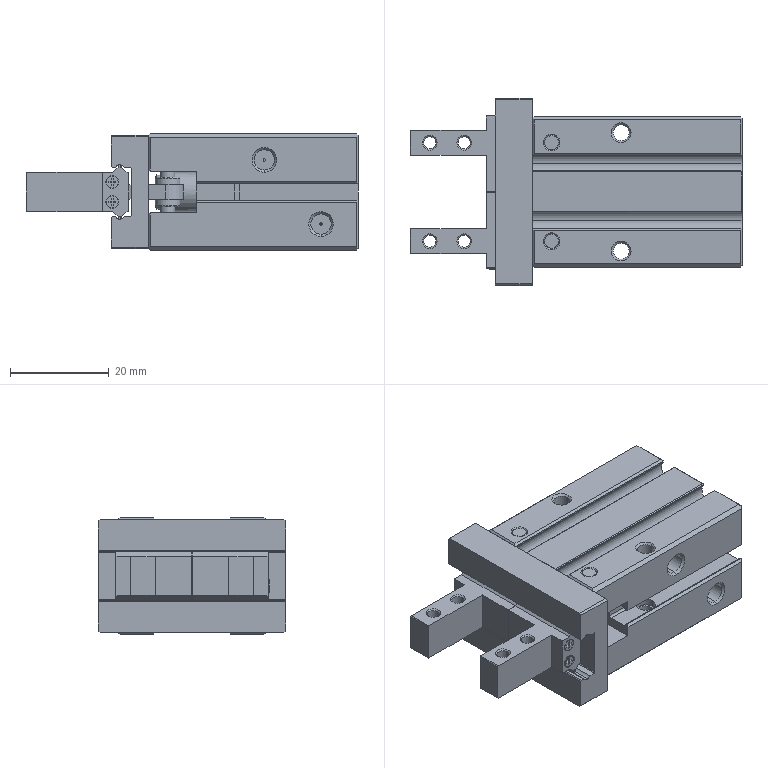Part | STEP file | HFZ16-B--BCL-H-21 | 1 solid | 467 faces | box 67.3 x 38 x 23.6 mm | volume 30878 mm3 | plane 234 | cylinder 157 | cone 68 | spline 8 | commonest cylinder face diameters 3.242 x16 0.8 x15 0.4 x14 0.6 x8 1 x8 2.4 x8